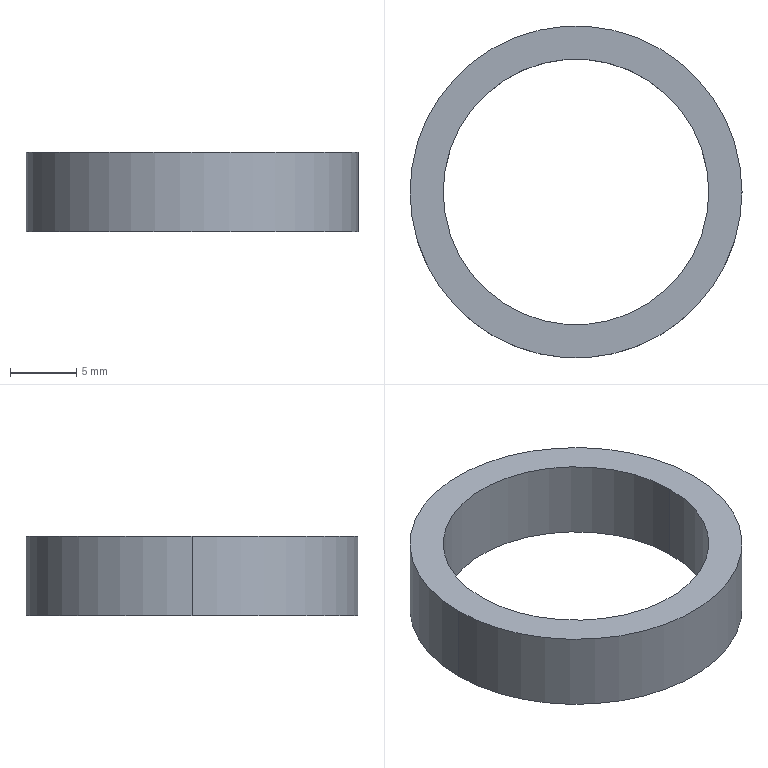Part | STEP file | X77-03307 | 1 solid | 6 faces | box 25 x 25 x 6 mm | volume 1060 mm3 | cylinder 4 | plane 2 | commonest cylinder face diameters 20 x2 25 x2
STEP:
#1=CARTESIAN_POINT('',(556.817,295.366,6.));
#2=VERTEX_POINT('',#1);
#3=CARTESIAN_POINT('',(576.817,295.366,6.));
#4=VERTEX_POINT('',#3);
#5=CARTESIAN_POINT('',(566.817,295.366,6.));
#6=DIRECTION('',(0.,0.,1.));
#7=DIRECTION('',(1.,0.,0.));
#8=AXIS2_PLACEMENT_3D('',#5,#6,#7);
#9=CIRCLE('',#8,10.);
#10=EDGE_CURVE('',#2,#4,#9,.T.);
#11=ORIENTED_EDGE('',*,*,#10,.T.);
#12=CARTESIAN_POINT('',(576.817,295.366,0.));
#13=VERTEX_POINT('',#12);
#14=CARTESIAN_POINT('',(576.817,295.366,6.));
#15=DIRECTION('',(0.,0.,-1.));
#16=VECTOR('',#15,1000.);
#17=LINE('',#14,#16);
#18=EDGE_CURVE('',#4,#13,#17,.T.);
#19=ORIENTED_EDGE('',*,*,#18,.T.);
#20=CARTESIAN_POINT('',(556.817,295.366,0.));
#21=VERTEX_POINT('',#20);
#22=CARTESIAN_POINT('',(566.817,295.366,0.));
#23=DIRECTION('',(0.,0.,1.));
#24=DIRECTION('',(1.,0.,0.));
#25=AXIS2_PLACEMENT_3D('',#22,#23,#24);
#26=CIRCLE('',#25,10.);
#27=EDGE_CURVE('',#21,#13,#26,.T.);
#28=ORIENTED_EDGE('',*,*,#27,.F.);
#29=CARTESIAN_POINT('',(556.817,295.366,6.));
#30=DIRECTION('',(0.,0.,-1.));
#31=VECTOR('',#30,1000.);
#32=LINE('',#29,#31);
#33=EDGE_CURVE('',#2,#21,#32,.T.);
#34=ORIENTED_EDGE('',*,*,#33,.F.);
#35=EDGE_LOOP('',(#11,#19,#28,#34));
#36=FACE_OUTER_BOUND('',#35,.T.);
#37=CARTESIAN_POINT('',(566.817,295.366,6.));
#38=DIRECTION('',(0.,0.,-1.));
#39=DIRECTION('',(-1.,0.,0.));
#40=AXIS2_PLACEMENT_3D('',#37,#38,#39);
#41=CYLINDRICAL_SURFACE('',#40,10.);
#42=ADVANCED_FACE('',(#36),#41,.F.);
#43=CARTESIAN_POINT('',(579.317,295.366,6.));
#44=VERTEX_POINT('',#43);
#45=CARTESIAN_POINT('',(554.317,295.366,6.));
#46=VERTEX_POINT('',#45);
#47=CARTESIAN_POINT('',(566.817,295.366,6.));
#48=DIRECTION('',(0.,0.,1.));
#49=DIRECTION('',(1.,0.,0.));
#50=AXIS2_PLACEMENT_3D('',#47,#48,#49);
#51=CIRCLE('',#50,12.5);
#52=EDGE_CURVE('',#44,#46,#51,.T.);
#53=ORIENTED_EDGE('',*,*,#52,.F.);
#54=CARTESIAN_POINT('',(579.317,295.366,0.));
#55=VERTEX_POINT('',#54);
#56=CARTESIAN_POINT('',(579.317,295.366,6.));
#57=DIRECTION('',(0.,0.,-1.));
#58=VECTOR('',#57,1000.);
#59=LINE('',#56,#58);
#60=EDGE_CURVE('',#44,#55,#59,.T.);
#61=ORIENTED_EDGE('',*,*,#60,.T.);
#62=CARTESIAN_POINT('',(554.317,295.366,0.));
#63=VERTEX_POINT('',#62);
#64=CARTESIAN_POINT('',(566.817,295.366,0.));
#65=DIRECTION('',(0.,0.,1.));
#66=DIRECTION('',(1.,0.,0.));
#67=AXIS2_PLACEMENT_3D('',#64,#65,#66);
#68=CIRCLE('',#67,12.5);
#69=EDGE_CURVE('',#55,#63,#68,.T.);
#70=ORIENTED_EDGE('',*,*,#69,.T.);
#71=CARTESIAN_POINT('',(554.317,295.366,6.));
#72=DIRECTION('',(0.,0.,-1.));
#73=VECTOR('',#72,1000.);
#74=LINE('',#71,#73);
#75=EDGE_CURVE('',#46,#63,#74,.T.);
#76=ORIENTED_EDGE('',*,*,#75,.F.);
#77=EDGE_LOOP('',(#53,#61,#70,#76));
#78=FACE_OUTER_BOUND('',#77,.T.);
#79=CARTESIAN_POINT('',(566.817,295.366,6.));
#80=DIRECTION('',(0.,0.,-1.));
#81=DIRECTION('',(-1.,0.,0.));
#82=AXIS2_PLACEMENT_3D('',#79,#80,#81);
#83=CYLINDRICAL_SURFACE('',#82,12.5);
#84=ADVANCED_FACE('',(#78),#83,.T.);
#85=CARTESIAN_POINT('',(566.817,295.366,6.));
#86=DIRECTION('',(0.,0.,1.));
#87=DIRECTION('',(1.,0.,0.));
#88=AXIS2_PLACEMENT_3D('',#85,#86,#87);
#89=CIRCLE('',#88,12.5);
#90=EDGE_CURVE('',#46,#44,#89,.T.);
#91=ORIENTED_EDGE('',*,*,#90,.T.);
#92=ORIENTED_EDGE('',*,*,#52,.T.);
#93=EDGE_LOOP('',(#91,#92));
#94=FACE_OUTER_BOUND('',#93,.T.);
#95=ORIENTED_EDGE('',*,*,#10,.F.);
#96=CARTESIAN_POINT('',(566.817,295.366,6.));
#97=DIRECTION('',(0.,0.,1.));
#98=DIRECTION('',(1.,0.,0.));
#99=AXIS2_PLACEMENT_3D('',#96,#97,#98);
#100=CIRCLE('',#99,10.);
#101=EDGE_CURVE('',#4,#2,#100,.T.);
#102=ORIENTED_EDGE('',*,*,#101,.F.);
#103=EDGE_LOOP('',(#95,#102));
#104=FACE_BOUND('',#103,.T.);
#105=CARTESIAN_POINT('',(566.817,295.366,6.));
#106=DIRECTION('',(0.,0.,1.));
#107=DIRECTION('',(1.,0.,0.));
#108=AXIS2_PLACEMENT_3D('',#105,#106,#107);
#109=PLANE('',#108);
#110=ADVANCED_FACE('',(#94,#104),#109,.T.);
#111=CARTESIAN_POINT('',(566.817,295.366,0.));
#112=DIRECTION('',(0.,0.,1.));
#113=DIRECTION('',(1.,0.,0.));
#114=AXIS2_PLACEMENT_3D('',#111,#112,#113);
#115=CIRCLE('',#114,12.5);
#116=EDGE_CURVE('',#63,#55,#115,.T.);
#117=ORIENTED_EDGE('',*,*,#116,.F.);
#118=ORIENTED_EDGE('',*,*,#69,.F.);
#119=EDGE_LOOP('',(#117,#118));
#120=FACE_OUTER_BOUND('',#119,.T.);
#121=ORIENTED_EDGE('',*,*,#27,.T.);
#122=CARTESIAN_POINT('',(566.817,295.366,0.));
#123=DIRECTION('',(0.,0.,1.));
#124=DIRECTION('',(1.,0.,0.));
#125=AXIS2_PLACEMENT_3D('',#122,#123,#124);
#126=CIRCLE('',#125,10.);
#127=EDGE_CURVE('',#13,#21,#126,.T.);
#128=ORIENTED_EDGE('',*,*,#127,.T.);
#129=EDGE_LOOP('',(#121,#128));
#130=FACE_BOUND('',#129,.T.);
#131=CARTESIAN_POINT('',(566.817,295.366,0.));
#132=DIRECTION('',(0.,0.,1.));
#133=DIRECTION('',(1.,0.,0.));
#134=AXIS2_PLACEMENT_3D('',#131,#132,#133);
#135=PLANE('',#134);
#136=ADVANCED_FACE('',(#120,#130),#135,.F.);
#137=ORIENTED_EDGE('',*,*,#60,.F.);
#138=ORIENTED_EDGE('',*,*,#90,.F.);
#139=ORIENTED_EDGE('',*,*,#75,.T.);
#140=ORIENTED_EDGE('',*,*,#116,.T.);
#141=EDGE_LOOP('',(#137,#138,#139,#140));
#142=FACE_OUTER_BOUND('',#141,.T.);
#143=CARTESIAN_POINT('',(566.817,295.366,6.));
#144=DIRECTION('',(0.,0.,-1.));
#145=DIRECTION('',(-1.,0.,0.));
#146=AXIS2_PLACEMENT_3D('',#143,#144,#145);
#147=CYLINDRICAL_SURFACE('',#146,12.5);
#148=ADVANCED_FACE('',(#142),#147,.T.);
#149=ORIENTED_EDGE('',*,*,#18,.F.);
#150=ORIENTED_EDGE('',*,*,#101,.T.);
#151=ORIENTED_EDGE('',*,*,#33,.T.);
#152=ORIENTED_EDGE('',*,*,#127,.F.);
#153=EDGE_LOOP('',(#149,#150,#151,#152));
#154=FACE_OUTER_BOUND('',#153,.T.);
#155=CARTESIAN_POINT('',(566.817,295.366,6.));
#156=DIRECTION('',(0.,0.,-1.));
#157=DIRECTION('',(-1.,0.,0.));
#158=AXIS2_PLACEMENT_3D('',#155,#156,#157);
#159=CYLINDRICAL_SURFACE('',#158,10.);
#160=ADVANCED_FACE('',(#154),#159,.F.);
#161=CLOSED_SHELL('',(#42,#84,#110,#136,#148,#160));
#162=MANIFOLD_SOLID_BREP('',#161);
#163=CARTESIAN_POINT('',(0.,0.,0.));
#164=DIRECTION('',(0.,0.,1.));
#165=DIRECTION('',(1.,0.,0.));
#166=AXIS2_PLACEMENT_3D('',#163,#164,#165);
#167=(LENGTH_UNIT()NAMED_UNIT(*)SI_UNIT(.MILLI.,.METRE.));
#168=UNCERTAINTY_MEASURE_WITH_UNIT(LENGTH_MEASURE(0.00001),#167,'','');
#169=(NAMED_UNIT(*)PLANE_ANGLE_UNIT()SI_UNIT($,.RADIAN.));
#170=(NAMED_UNIT(*)SI_UNIT($,.STERADIAN.)SOLID_ANGLE_UNIT());
#171=(GEOMETRIC_REPRESENTATION_CONTEXT(3)GLOBAL_UNCERTAINTY_ASSIGNED_CONTEXT((#168))GLOBAL_UNIT_ASSIGNED_CONTEXT((#167,#169,#170))REPRESENTATION_CONTEXT('',''));
#172=ADVANCED_BREP_SHAPE_REPRESENTATION('',(#162,#166),#171);